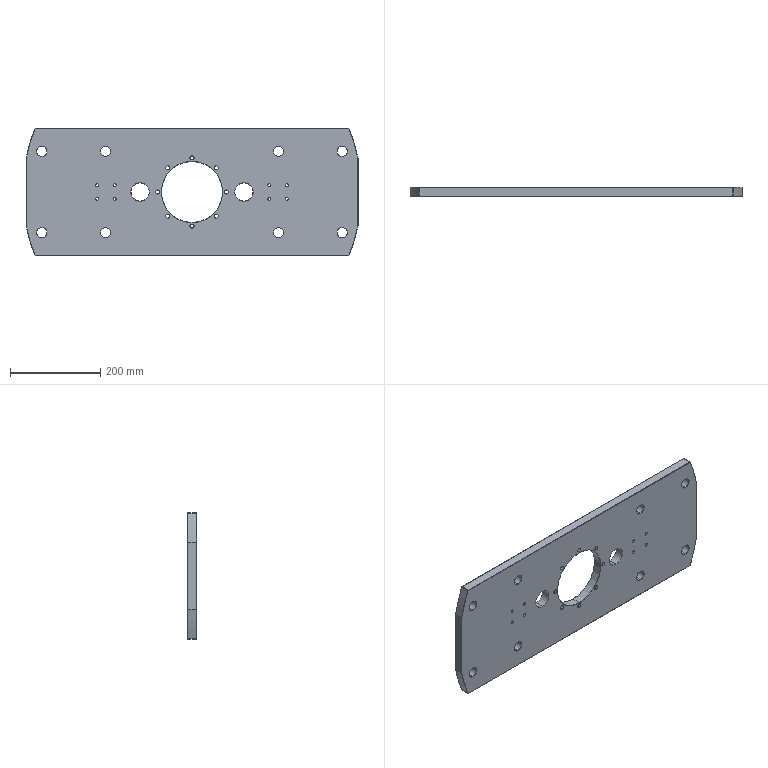Part | SolidWorks | features HoleWzd 3, MirrorPattern 3, ICE 2, Chamfer 1, Cut 1, Extrusion 1 | 1 solid | 160 faces | box 735 x 20 x 280 mm | volume 3653235 mm3 | cylinder 74 | cone 52 | plane 34 | commonest cylinder face diameters 6.6 x16 9 x16 11 x16 22 x16 40 x4 750 x4